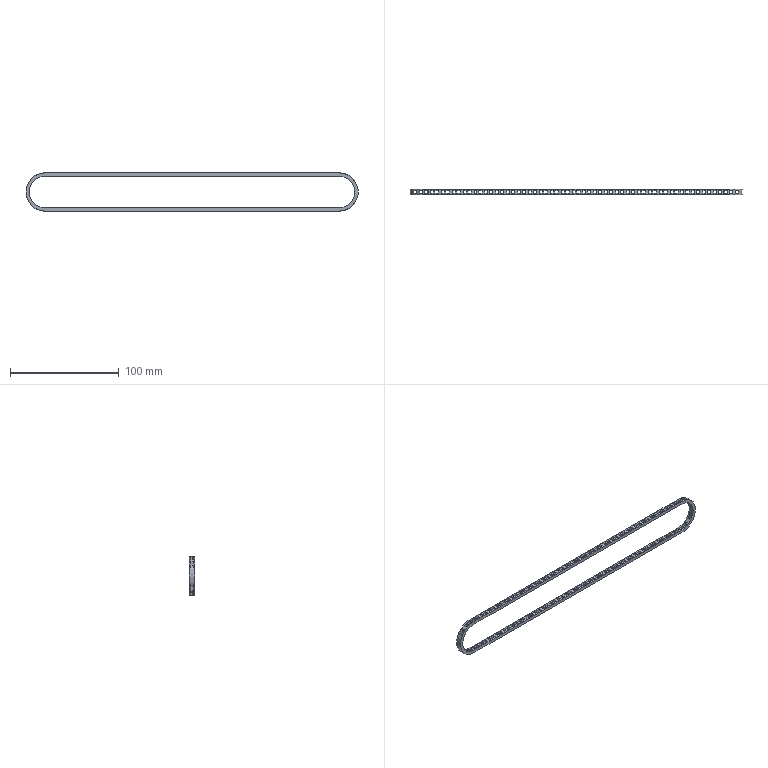Part | STEP file | 1/4in long chain | 1 solid | 490 faces | box 305 x 5 x 35 mm | volume 6649 mm3 | plane 486 | cylinder 4 | commonest cylinder face diameters 29 x2 35 x2